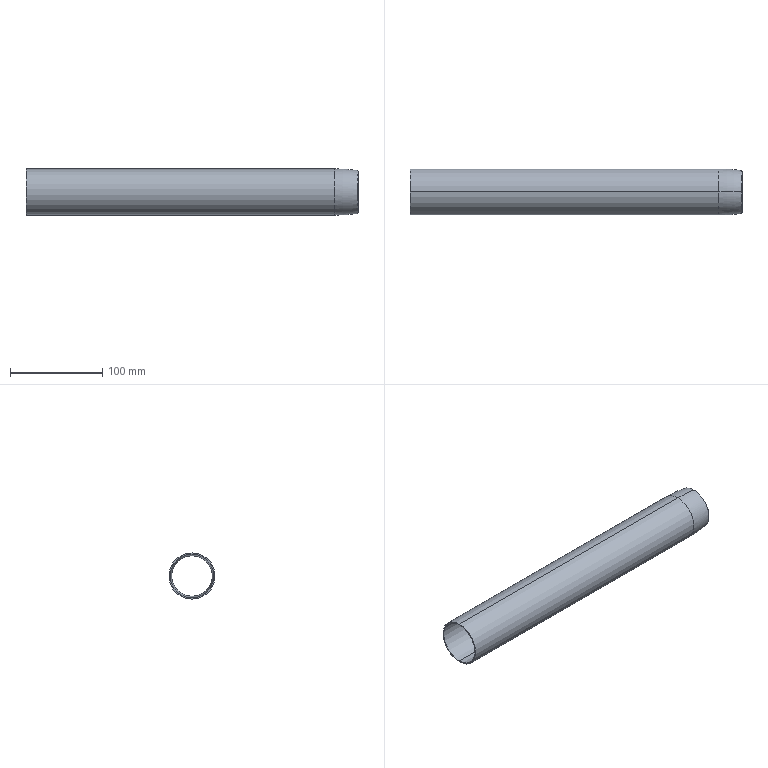Part | SolidWorks | features BaseBody 1 | 1 solid | 12 faces | box 359.5 x 50 x 50 mm | volume 66032 mm3 | torus 6 | cylinder 4 | plane 2 | commonest cylinder face diameters 47.6 x2 50 x2
STEP:
#1=CARTESIAN_POINT('',(334.5,0.,-23.8));
#2=VERTEX_POINT('',#1);
#3=CARTESIAN_POINT('',(334.5,0.,23.8));
#4=VERTEX_POINT('',#3);
#5=CARTESIAN_POINT('',(334.5,0.,0.));
#6=DIRECTION('',(-1.,0.,0.));
#7=DIRECTION('',(0.,0.,1.));
#8=AXIS2_PLACEMENT_3D('',#5,#6,#7);
#9=CIRCLE('',#8,23.8);
#10=EDGE_CURVE('',#2,#4,#9,.T.);
#11=ORIENTED_EDGE('',*,*,#10,.F.);
#12=CARTESIAN_POINT('',(0.,0.,-23.8));
#13=VERTEX_POINT('',#12);
#14=CARTESIAN_POINT('',(0.,0.,-23.8));
#15=DIRECTION('',(-1.,0.,0.));
#16=VECTOR('',#15,1000.);
#17=LINE('',#14,#16);
#18=EDGE_CURVE('',#2,#13,#17,.T.);
#19=ORIENTED_EDGE('',*,*,#18,.T.);
#20=CARTESIAN_POINT('',(0.,0.,23.8));
#21=VERTEX_POINT('',#20);
#22=CARTESIAN_POINT('',(0.,0.,0.));
#23=DIRECTION('',(-1.,0.,0.));
#24=DIRECTION('',(0.,0.,-1.));
#25=AXIS2_PLACEMENT_3D('',#22,#23,#24);
#26=CIRCLE('',#25,23.8);
#27=EDGE_CURVE('',#13,#21,#26,.T.);
#28=ORIENTED_EDGE('',*,*,#27,.T.);
#29=CARTESIAN_POINT('',(0.,0.,23.8));
#30=DIRECTION('',(-1.,0.,0.));
#31=VECTOR('',#30,1000.);
#32=LINE('',#29,#31);
#33=EDGE_CURVE('',#4,#21,#32,.T.);
#34=ORIENTED_EDGE('',*,*,#33,.F.);
#35=EDGE_LOOP('',(#11,#19,#28,#34));
#36=FACE_OUTER_BOUND('',#35,.T.);
#37=CARTESIAN_POINT('',(0.,0.,0.));
#38=DIRECTION('',(-1.,0.,0.));
#39=DIRECTION('',(0.,0.,1.));
#40=AXIS2_PLACEMENT_3D('',#37,#38,#39);
#41=CYLINDRICAL_SURFACE('',#40,23.8);
#42=ADVANCED_FACE('',(#36),#41,.F.);
#43=CARTESIAN_POINT('',(359.5,0.,-21.938));
#44=VERTEX_POINT('',#43);
#45=CARTESIAN_POINT('',(359.5,0.,21.938));
#46=VERTEX_POINT('',#45);
#47=CARTESIAN_POINT('',(359.5,0.,0.));
#48=DIRECTION('',(-1.,0.,0.));
#49=DIRECTION('',(0.,0.,1.));
#50=AXIS2_PLACEMENT_3D('',#47,#48,#49);
#51=CIRCLE('',#50,21.938);
#52=EDGE_CURVE('',#44,#46,#51,.T.);
#53=ORIENTED_EDGE('',*,*,#52,.F.);
#54=CARTESIAN_POINT('',(334.5,0.,145.));
#55=DIRECTION('',(0.,1.,0.));
#56=DIRECTION('',(0.,0.,1.));
#57=AXIS2_PLACEMENT_3D('',#54,#55,#56);
#58=CIRCLE('',#57,168.8);
#59=EDGE_CURVE('',#44,#2,#58,.T.);
#60=ORIENTED_EDGE('',*,*,#59,.T.);
#61=ORIENTED_EDGE('',*,*,#10,.T.);
#62=CARTESIAN_POINT('',(334.5,0.,-145.));
#63=DIRECTION('',(0.,-1.,0.));
#64=DIRECTION('',(0.,0.,-1.));
#65=AXIS2_PLACEMENT_3D('',#62,#63,#64);
#66=CIRCLE('',#65,168.8);
#67=EDGE_CURVE('',#46,#4,#66,.T.);
#68=ORIENTED_EDGE('',*,*,#67,.F.);
#69=EDGE_LOOP('',(#53,#60,#61,#68));
#70=FACE_OUTER_BOUND('',#69,.T.);
#71=CARTESIAN_POINT('',(334.5,0.,0.));
#72=DIRECTION('',(-1.,0.,0.));
#73=DIRECTION('',(0.,0.,1.));
#74=AXIS2_PLACEMENT_3D('',#71,#72,#73);
#75=TOROIDAL_SURFACE('',#74,-145.,168.8);
#76=ADVANCED_FACE('',(#70),#75,.F.);
#77=CARTESIAN_POINT('',(334.5,0.,25.));
#78=VERTEX_POINT('',#77);
#79=CARTESIAN_POINT('',(334.5,0.,-25.));
#80=VERTEX_POINT('',#79);
#81=CARTESIAN_POINT('',(334.5,0.,0.));
#82=DIRECTION('',(-1.,0.,0.));
#83=DIRECTION('',(0.,0.,1.));
#84=AXIS2_PLACEMENT_3D('',#81,#82,#83);
#85=CIRCLE('',#84,25.);
#86=EDGE_CURVE('',#78,#80,#85,.T.);
#87=ORIENTED_EDGE('',*,*,#86,.T.);
#88=CARTESIAN_POINT('',(0.,0.,-25.));
#89=VERTEX_POINT('',#88);
#90=CARTESIAN_POINT('',(0.,0.,-25.));
#91=DIRECTION('',(-1.,0.,0.));
#92=VECTOR('',#91,1000.);
#93=LINE('',#90,#92);
#94=EDGE_CURVE('',#80,#89,#93,.T.);
#95=ORIENTED_EDGE('',*,*,#94,.T.);
#96=CARTESIAN_POINT('',(0.,0.,25.));
#97=VERTEX_POINT('',#96);
#98=CARTESIAN_POINT('',(0.,0.,0.));
#99=DIRECTION('',(-1.,0.,0.));
#100=DIRECTION('',(0.,0.,1.));
#101=AXIS2_PLACEMENT_3D('',#98,#99,#100);
#102=CIRCLE('',#101,25.);
#103=EDGE_CURVE('',#97,#89,#102,.T.);
#104=ORIENTED_EDGE('',*,*,#103,.F.);
#105=CARTESIAN_POINT('',(0.,0.,25.));
#106=DIRECTION('',(-1.,0.,0.));
#107=VECTOR('',#106,1000.);
#108=LINE('',#105,#107);
#109=EDGE_CURVE('',#78,#97,#108,.T.);
#110=ORIENTED_EDGE('',*,*,#109,.F.);
#111=EDGE_LOOP('',(#87,#95,#104,#110));
#112=FACE_OUTER_BOUND('',#111,.T.);
#113=CARTESIAN_POINT('',(0.,0.,0.));
#114=DIRECTION('',(-1.,0.,0.));
#115=DIRECTION('',(0.,0.,1.));
#116=AXIS2_PLACEMENT_3D('',#113,#114,#115);
#117=CYLINDRICAL_SURFACE('',#116,25.);
#118=ADVANCED_FACE('',(#112),#117,.T.);
#119=CARTESIAN_POINT('',(359.072,0.,23.215));
#120=VERTEX_POINT('',#119);
#121=CARTESIAN_POINT('',(359.072,0.,-23.215));
#122=VERTEX_POINT('',#121);
#123=CARTESIAN_POINT('',(359.072,0.,0.));
#124=DIRECTION('',(-1.,0.,0.));
#125=DIRECTION('',(0.,0.,1.));
#126=AXIS2_PLACEMENT_3D('',#123,#124,#125);
#127=CIRCLE('',#126,23.215);
#128=EDGE_CURVE('',#120,#122,#127,.T.);
#129=ORIENTED_EDGE('',*,*,#128,.T.);
#130=CARTESIAN_POINT('',(334.5,0.,145.));
#131=DIRECTION('',(0.,1.,0.));
#132=DIRECTION('',(0.,0.,1.));
#133=AXIS2_PLACEMENT_3D('',#130,#131,#132);
#134=CIRCLE('',#133,170.);
#135=EDGE_CURVE('',#122,#80,#134,.T.);
#136=ORIENTED_EDGE('',*,*,#135,.T.);
#137=ORIENTED_EDGE('',*,*,#86,.F.);
#138=CARTESIAN_POINT('',(334.5,0.,-145.));
#139=DIRECTION('',(0.,-1.,0.));
#140=DIRECTION('',(0.,0.,-1.));
#141=AXIS2_PLACEMENT_3D('',#138,#139,#140);
#142=CIRCLE('',#141,170.);
#143=EDGE_CURVE('',#120,#78,#142,.T.);
#144=ORIENTED_EDGE('',*,*,#143,.F.);
#145=EDGE_LOOP('',(#129,#136,#137,#144));
#146=FACE_OUTER_BOUND('',#145,.T.);
#147=CARTESIAN_POINT('',(334.5,0.,0.));
#148=DIRECTION('',(-1.,0.,0.));
#149=DIRECTION('',(0.,0.,1.));
#150=AXIS2_PLACEMENT_3D('',#147,#148,#149);
#151=TOROIDAL_SURFACE('',#150,-145.,170.);
#152=ADVANCED_FACE('',(#146),#151,.T.);
#153=CARTESIAN_POINT('',(359.5,0.,22.72));
#154=VERTEX_POINT('',#153);
#155=CARTESIAN_POINT('',(359.5,0.,-22.72));
#156=VERTEX_POINT('',#155);
#157=CARTESIAN_POINT('',(359.5,0.,0.));
#158=DIRECTION('',(-1.,0.,0.));
#159=DIRECTION('',(0.,0.,1.));
#160=AXIS2_PLACEMENT_3D('',#157,#158,#159);
#161=CIRCLE('',#160,22.72);
#162=EDGE_CURVE('',#154,#156,#161,.T.);
#163=ORIENTED_EDGE('',*,*,#162,.T.);
#164=CARTESIAN_POINT('',(359.,0.,-22.72));
#165=DIRECTION('',(0.,1.,0.));
#166=DIRECTION('',(0.,0.,1.));
#167=AXIS2_PLACEMENT_3D('',#164,#165,#166);
#168=CIRCLE('',#167,0.5);
#169=EDGE_CURVE('',#156,#122,#168,.T.);
#170=ORIENTED_EDGE('',*,*,#169,.T.);
#171=ORIENTED_EDGE('',*,*,#128,.F.);
#172=CARTESIAN_POINT('',(359.,0.,22.72));
#173=DIRECTION('',(0.,-1.,0.));
#174=DIRECTION('',(0.,0.,-1.));
#175=AXIS2_PLACEMENT_3D('',#172,#173,#174);
#176=CIRCLE('',#175,0.5);
#177=EDGE_CURVE('',#154,#120,#176,.T.);
#178=ORIENTED_EDGE('',*,*,#177,.F.);
#179=EDGE_LOOP('',(#163,#170,#171,#178));
#180=FACE_OUTER_BOUND('',#179,.T.);
#181=CARTESIAN_POINT('',(359.,0.,0.));
#182=DIRECTION('',(-1.,0.,0.));
#183=DIRECTION('',(0.,0.,1.));
#184=AXIS2_PLACEMENT_3D('',#181,#182,#183);
#185=TOROIDAL_SURFACE('',#184,22.72,0.5);
#186=ADVANCED_FACE('',(#180),#185,.T.);
#187=CARTESIAN_POINT('',(359.5,0.,0.));
#188=DIRECTION('',(-1.,0.,0.));
#189=DIRECTION('',(0.,0.,1.));
#190=AXIS2_PLACEMENT_3D('',#187,#188,#189);
#191=CIRCLE('',#190,21.938);
#192=EDGE_CURVE('',#46,#44,#191,.T.);
#193=ORIENTED_EDGE('',*,*,#192,.T.);
#194=ORIENTED_EDGE('',*,*,#52,.T.);
#195=EDGE_LOOP('',(#193,#194));
#196=FACE_BOUND('',#195,.T.);
#197=ORIENTED_EDGE('',*,*,#162,.F.);
#198=CARTESIAN_POINT('',(359.5,0.,0.));
#199=DIRECTION('',(-1.,0.,0.));
#200=DIRECTION('',(0.,0.,1.));
#201=AXIS2_PLACEMENT_3D('',#198,#199,#200);
#202=CIRCLE('',#201,22.72);
#203=EDGE_CURVE('',#156,#154,#202,.T.);
#204=ORIENTED_EDGE('',*,*,#203,.F.);
#205=EDGE_LOOP('',(#197,#204));
#206=FACE_OUTER_BOUND('',#205,.T.);
#207=CARTESIAN_POINT('',(359.5,22.72,0.));
#208=DIRECTION('',(-1.,0.,0.));
#209=DIRECTION('',(0.,0.,1.));
#210=AXIS2_PLACEMENT_3D('',#207,#208,#209);
#211=PLANE('',#210);
#212=ADVANCED_FACE('',(#196,#206),#211,.F.);
#213=ORIENTED_EDGE('',*,*,#169,.F.);
#214=ORIENTED_EDGE('',*,*,#203,.T.);
#215=ORIENTED_EDGE('',*,*,#177,.T.);
#216=CARTESIAN_POINT('',(359.072,0.,0.));
#217=DIRECTION('',(-1.,0.,0.));
#218=DIRECTION('',(0.,0.,1.));
#219=AXIS2_PLACEMENT_3D('',#216,#217,#218);
#220=CIRCLE('',#219,23.215);
#221=EDGE_CURVE('',#122,#120,#220,.T.);
#222=ORIENTED_EDGE('',*,*,#221,.F.);
#223=EDGE_LOOP('',(#213,#214,#215,#222));
#224=FACE_OUTER_BOUND('',#223,.T.);
#225=CARTESIAN_POINT('',(359.,0.,0.));
#226=DIRECTION('',(-1.,0.,0.));
#227=DIRECTION('',(0.,0.,1.));
#228=AXIS2_PLACEMENT_3D('',#225,#226,#227);
#229=TOROIDAL_SURFACE('',#228,22.72,0.5);
#230=ADVANCED_FACE('',(#224),#229,.T.);
#231=ORIENTED_EDGE('',*,*,#135,.F.);
#232=ORIENTED_EDGE('',*,*,#221,.T.);
#233=ORIENTED_EDGE('',*,*,#143,.T.);
#234=CARTESIAN_POINT('',(334.5,0.,0.));
#235=DIRECTION('',(-1.,0.,0.));
#236=DIRECTION('',(0.,0.,1.));
#237=AXIS2_PLACEMENT_3D('',#234,#235,#236);
#238=CIRCLE('',#237,25.);
#239=EDGE_CURVE('',#80,#78,#238,.T.);
#240=ORIENTED_EDGE('',*,*,#239,.F.);
#241=EDGE_LOOP('',(#231,#232,#233,#240));
#242=FACE_OUTER_BOUND('',#241,.T.);
#243=CARTESIAN_POINT('',(334.5,0.,0.));
#244=DIRECTION('',(-1.,0.,0.));
#245=DIRECTION('',(0.,0.,1.));
#246=AXIS2_PLACEMENT_3D('',#243,#244,#245);
#247=TOROIDAL_SURFACE('',#246,-145.,170.);
#248=ADVANCED_FACE('',(#242),#247,.T.);
#249=ORIENTED_EDGE('',*,*,#94,.F.);
#250=ORIENTED_EDGE('',*,*,#239,.T.);
#251=ORIENTED_EDGE('',*,*,#109,.T.);
#252=CARTESIAN_POINT('',(0.,0.,0.));
#253=DIRECTION('',(-1.,0.,0.));
#254=DIRECTION('',(0.,0.,1.));
#255=AXIS2_PLACEMENT_3D('',#252,#253,#254);
#256=CIRCLE('',#255,25.);
#257=EDGE_CURVE('',#89,#97,#256,.T.);
#258=ORIENTED_EDGE('',*,*,#257,.F.);
#259=EDGE_LOOP('',(#249,#250,#251,#258));
#260=FACE_OUTER_BOUND('',#259,.T.);
#261=CARTESIAN_POINT('',(0.,0.,0.));
#262=DIRECTION('',(-1.,0.,0.));
#263=DIRECTION('',(0.,0.,1.));
#264=AXIS2_PLACEMENT_3D('',#261,#262,#263);
#265=CYLINDRICAL_SURFACE('',#264,25.);
#266=ADVANCED_FACE('',(#260),#265,.T.);
#267=CARTESIAN_POINT('',(0.,0.,0.));
#268=DIRECTION('',(-1.,0.,0.));
#269=DIRECTION('',(0.,0.,-1.));
#270=AXIS2_PLACEMENT_3D('',#267,#268,#269);
#271=CIRCLE('',#270,23.8);
#272=EDGE_CURVE('',#21,#13,#271,.T.);
#273=ORIENTED_EDGE('',*,*,#272,.F.);
#274=ORIENTED_EDGE('',*,*,#27,.F.);
#275=EDGE_LOOP('',(#273,#274));
#276=FACE_BOUND('',#275,.T.);
#277=ORIENTED_EDGE('',*,*,#103,.T.);
#278=ORIENTED_EDGE('',*,*,#257,.T.);
#279=EDGE_LOOP('',(#277,#278));
#280=FACE_OUTER_BOUND('',#279,.T.);
#281=CARTESIAN_POINT('',(0.,0.,0.));
#282=DIRECTION('',(1.,0.,0.));
#283=DIRECTION('',(0.,0.,-1.));
#284=AXIS2_PLACEMENT_3D('',#281,#282,#283);
#285=PLANE('',#284);
#286=ADVANCED_FACE('',(#276,#280),#285,.F.);
#287=ORIENTED_EDGE('',*,*,#59,.F.);
#288=ORIENTED_EDGE('',*,*,#192,.F.);
#289=ORIENTED_EDGE('',*,*,#67,.T.);
#290=CARTESIAN_POINT('',(334.5,0.,0.));
#291=DIRECTION('',(-1.,0.,0.));
#292=DIRECTION('',(0.,0.,1.));
#293=AXIS2_PLACEMENT_3D('',#290,#291,#292);
#294=CIRCLE('',#293,23.8);
#295=EDGE_CURVE('',#4,#2,#294,.T.);
#296=ORIENTED_EDGE('',*,*,#295,.T.);
#297=EDGE_LOOP('',(#287,#288,#289,#296));
#298=FACE_OUTER_BOUND('',#297,.T.);
#299=CARTESIAN_POINT('',(334.5,0.,0.));
#300=DIRECTION('',(-1.,0.,0.));
#301=DIRECTION('',(0.,0.,1.));
#302=AXIS2_PLACEMENT_3D('',#299,#300,#301);
#303=TOROIDAL_SURFACE('',#302,-145.,168.8);
#304=ADVANCED_FACE('',(#298),#303,.F.);
#305=ORIENTED_EDGE('',*,*,#18,.F.);
#306=ORIENTED_EDGE('',*,*,#295,.F.);
#307=ORIENTED_EDGE('',*,*,#33,.T.);
#308=ORIENTED_EDGE('',*,*,#272,.T.);
#309=EDGE_LOOP('',(#305,#306,#307,#308));
#310=FACE_OUTER_BOUND('',#309,.T.);
#311=CARTESIAN_POINT('',(0.,0.,0.));
#312=DIRECTION('',(-1.,0.,0.));
#313=DIRECTION('',(0.,0.,1.));
#314=AXIS2_PLACEMENT_3D('',#311,#312,#313);
#315=CYLINDRICAL_SURFACE('',#314,23.8);
#316=ADVANCED_FACE('',(#310),#315,.F.);
#317=CLOSED_SHELL('',(#42,#76,#118,#152,#186,#212,#230,#248,#266,#286,#304,#316));
#318=MANIFOLD_SOLID_BREP('',#317);
#319=CARTESIAN_POINT('',(0.,0.,0.));
#320=DIRECTION('',(0.,0.,1.));
#321=DIRECTION('',(1.,0.,0.));
#322=AXIS2_PLACEMENT_3D('',#319,#320,#321);
#323=(LENGTH_UNIT()NAMED_UNIT(*)SI_UNIT(.MILLI.,.METRE.));
#324=UNCERTAINTY_MEASURE_WITH_UNIT(LENGTH_MEASURE(0.00001),#323,'','');
#325=(NAMED_UNIT(*)PLANE_ANGLE_UNIT()SI_UNIT($,.RADIAN.));
#326=(NAMED_UNIT(*)SI_UNIT($,.STERADIAN.)SOLID_ANGLE_UNIT());
#327=(GEOMETRIC_REPRESENTATION_CONTEXT(3)GLOBAL_UNCERTAINTY_ASSIGNED_CONTEXT((#324))GLOBAL_UNIT_ASSIGNED_CONTEXT((#323,#325,#326))REPRESENTATION_CONTEXT('',''));
#328=ADVANCED_BREP_SHAPE_REPRESENTATION('',(#318,#322),#327);